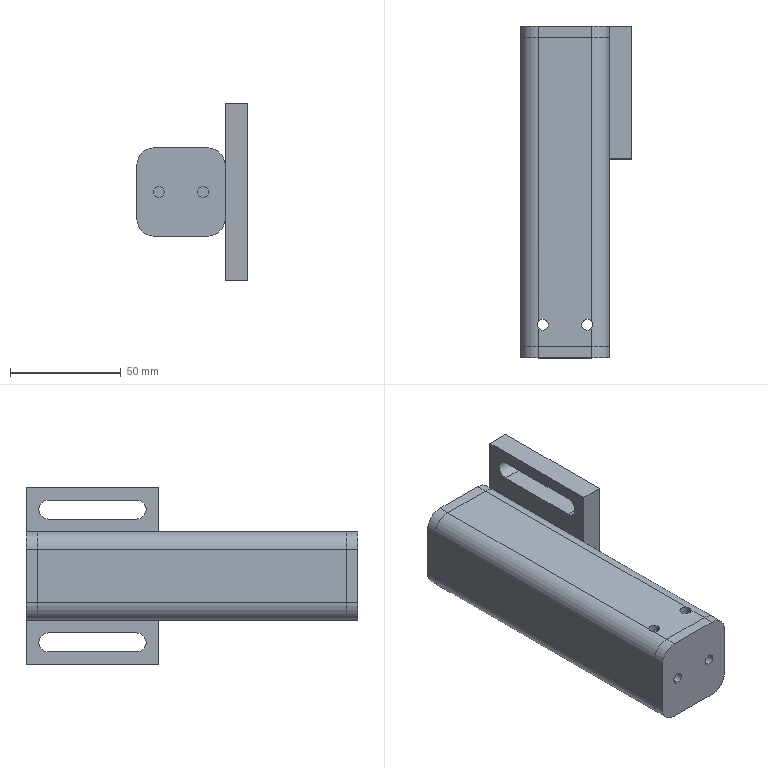Part | SolidWorks | features EndCap 2, HoleWzd 2, ICE 2, WeldMemberFeat 1, WeldmentFeature 1 | 4 solids | 64 faces | box 50 x 150 x 80 mm | volume 129877 mm3 | plane 32 | cylinder 32 | commonest cylinder face diameters 5 x12 16 x12 8 x4 8.5 x4